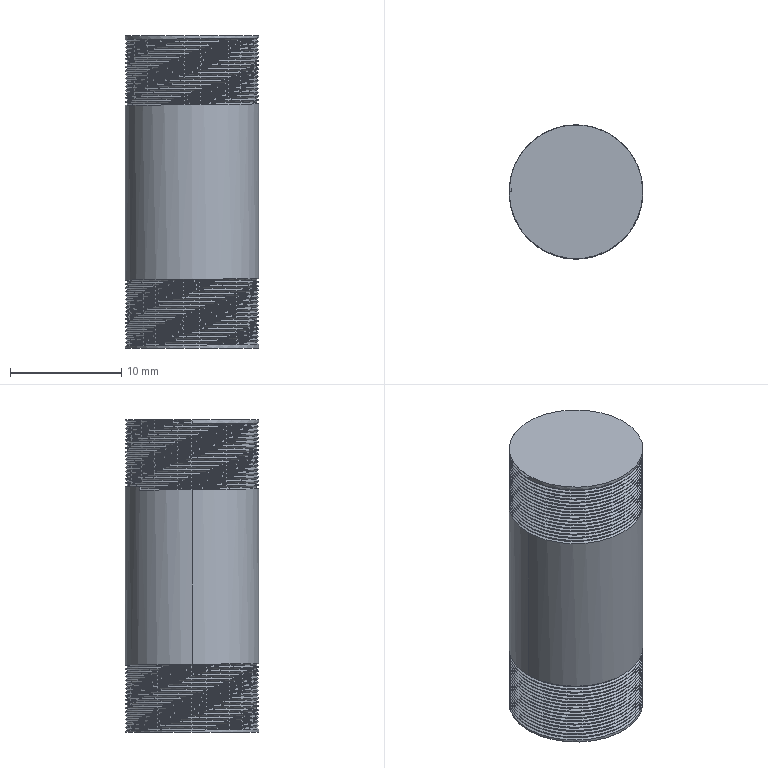Part | STEP file | Hinge seat cylinder | 1 solid | 82 faces | box 12 x 12 x 28 mm | volume 3114 mm3 | cylinder 70 | plane 6 | spline 6 | commonest cylinder face diameters 12 x70